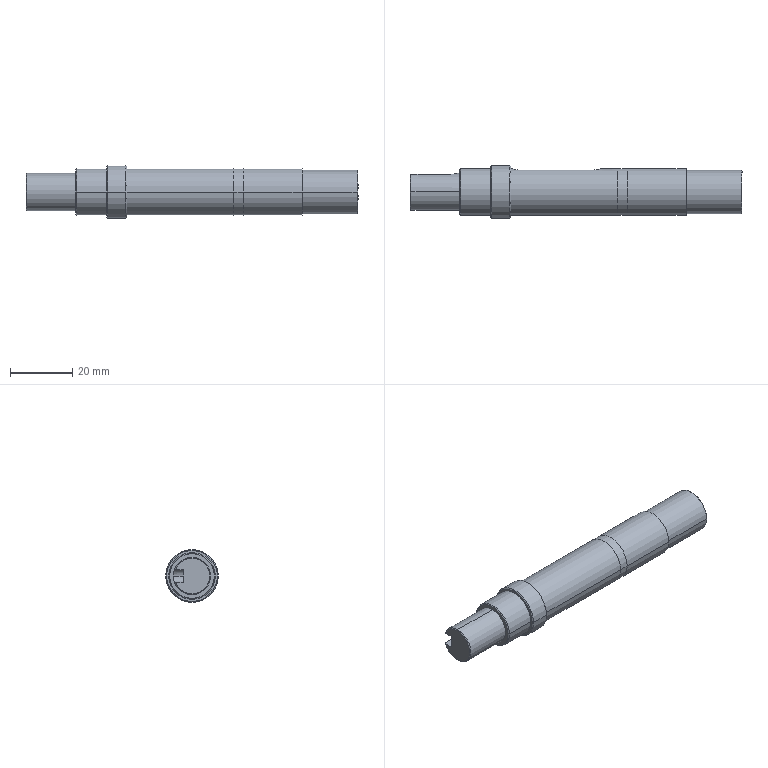Part | NX | 1 solid | 40 faces | box 107 x 17 x 17 mm | volume 17288 mm3 | cylinder 19 | plane 12 | cone 9 | commonest cylinder face diameters 15 x8 5 x3 4 x2 12 x2 14 x2 17 x2